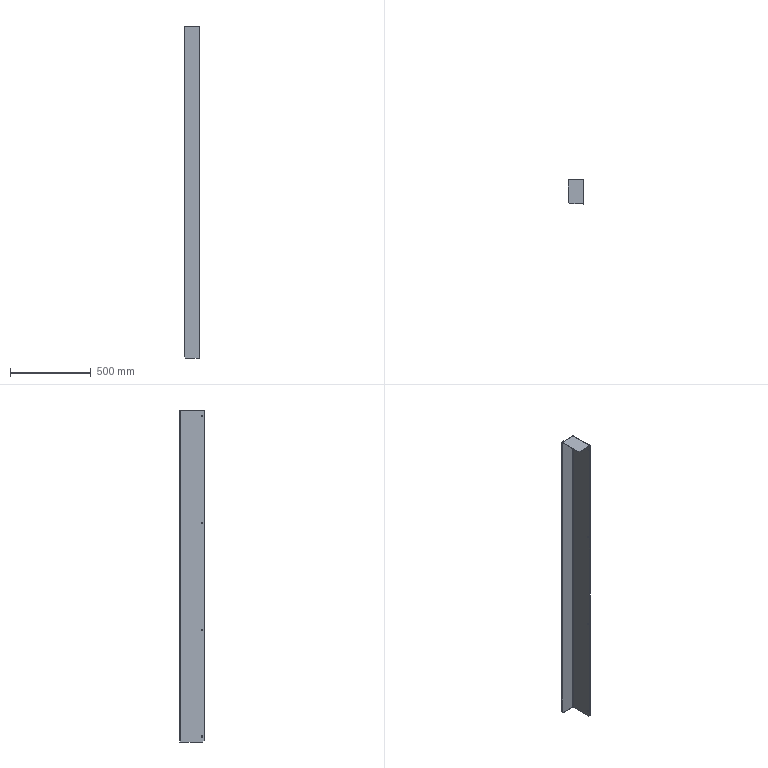Part | STEP file | HXGR200008-05-04 | 2 solids | 32 faces | box 98 x 150 x 2052 mm | volume 1030227 mm3 | plane 22 | cylinder 10 | commonest cylinder face diameters 8 x8 6 x1 10 x1
STEP:
#1=CARTESIAN_POINT('',(96.,-136.,332.));
#2=VERTEX_POINT('',#1);
#3=CARTESIAN_POINT('',(96.,-136.,324.));
#4=VERTEX_POINT('',#3);
#5=CARTESIAN_POINT('',(96.,-136.,328.));
#6=DIRECTION('',(1.,0.,0.));
#7=DIRECTION('',(0.,1.,0.));
#8=AXIS2_PLACEMENT_3D('',#5,#6,#7);
#9=CIRCLE('',#8,4.);
#10=EDGE_CURVE('',#2,#4,#9,.T.);
#11=ORIENTED_EDGE('',*,*,#10,.F.);
#12=CARTESIAN_POINT('',(98.,-136.,332.));
#13=VERTEX_POINT('',#12);
#14=CARTESIAN_POINT('',(98.,-136.,332.));
#15=DIRECTION('',(1.,0.,0.));
#16=VECTOR('',#15,1000.);
#17=LINE('',#14,#16);
#18=EDGE_CURVE('',#2,#13,#17,.T.);
#19=ORIENTED_EDGE('',*,*,#18,.T.);
#20=CARTESIAN_POINT('',(98.,-136.,324.));
#21=VERTEX_POINT('',#20);
#22=CARTESIAN_POINT('',(98.,-136.,328.));
#23=DIRECTION('',(1.,0.,0.));
#24=DIRECTION('',(0.,0.,-1.));
#25=AXIS2_PLACEMENT_3D('',#22,#23,#24);
#26=CIRCLE('',#25,4.);
#27=EDGE_CURVE('',#13,#21,#26,.T.);
#28=ORIENTED_EDGE('',*,*,#27,.T.);
#29=CARTESIAN_POINT('',(98.,-136.,324.));
#30=DIRECTION('',(1.,0.,0.));
#31=VECTOR('',#30,1000.);
#32=LINE('',#29,#31);
#33=EDGE_CURVE('',#4,#21,#32,.T.);
#34=ORIENTED_EDGE('',*,*,#33,.F.);
#35=EDGE_LOOP('',(#11,#19,#28,#34));
#36=FACE_OUTER_BOUND('',#35,.T.);
#37=CARTESIAN_POINT('',(98.,-136.,328.));
#38=DIRECTION('',(1.,0.,0.));
#39=DIRECTION('',(0.,0.,-1.));
#40=AXIS2_PLACEMENT_3D('',#37,#38,#39);
#41=CYLINDRICAL_SURFACE('',#40,4.);
#42=ADVANCED_FACE('',(#36),#41,.F.);
#43=CARTESIAN_POINT('',(96.,-136.,-328.));
#44=VERTEX_POINT('',#43);
#45=CARTESIAN_POINT('',(96.,-136.,-336.));
#46=VERTEX_POINT('',#45);
#47=CARTESIAN_POINT('',(96.,-136.,-332.));
#48=DIRECTION('',(1.,0.,0.));
#49=DIRECTION('',(0.,1.,0.));
#50=AXIS2_PLACEMENT_3D('',#47,#48,#49);
#51=CIRCLE('',#50,4.);
#52=EDGE_CURVE('',#44,#46,#51,.T.);
#53=ORIENTED_EDGE('',*,*,#52,.F.);
#54=CARTESIAN_POINT('',(98.,-136.,-328.));
#55=VERTEX_POINT('',#54);
#56=CARTESIAN_POINT('',(98.,-136.,-328.));
#57=DIRECTION('',(1.,0.,0.));
#58=VECTOR('',#57,1000.);
#59=LINE('',#56,#58);
#60=EDGE_CURVE('',#44,#55,#59,.T.);
#61=ORIENTED_EDGE('',*,*,#60,.T.);
#62=CARTESIAN_POINT('',(98.,-136.,-336.));
#63=VERTEX_POINT('',#62);
#64=CARTESIAN_POINT('',(98.,-136.,-332.));
#65=DIRECTION('',(1.,0.,0.));
#66=DIRECTION('',(0.,0.,-1.));
#67=AXIS2_PLACEMENT_3D('',#64,#65,#66);
#68=CIRCLE('',#67,4.);
#69=EDGE_CURVE('',#55,#63,#68,.T.);
#70=ORIENTED_EDGE('',*,*,#69,.T.);
#71=CARTESIAN_POINT('',(98.,-136.,-336.));
#72=DIRECTION('',(1.,0.,0.));
#73=VECTOR('',#72,1000.);
#74=LINE('',#71,#73);
#75=EDGE_CURVE('',#46,#63,#74,.T.);
#76=ORIENTED_EDGE('',*,*,#75,.F.);
#77=EDGE_LOOP('',(#53,#61,#70,#76));
#78=FACE_OUTER_BOUND('',#77,.T.);
#79=CARTESIAN_POINT('',(98.,-136.,-332.));
#80=DIRECTION('',(1.,0.,0.));
#81=DIRECTION('',(0.,0.,-1.));
#82=AXIS2_PLACEMENT_3D('',#79,#80,#81);
#83=CYLINDRICAL_SURFACE('',#82,4.);
#84=ADVANCED_FACE('',(#78),#83,.F.);
#85=CARTESIAN_POINT('',(96.,-136.,-988.));
#86=VERTEX_POINT('',#85);
#87=CARTESIAN_POINT('',(96.,-136.,-996.));
#88=VERTEX_POINT('',#87);
#89=CARTESIAN_POINT('',(96.,-136.,-992.));
#90=DIRECTION('',(1.,0.,0.));
#91=DIRECTION('',(0.,1.,0.));
#92=AXIS2_PLACEMENT_3D('',#89,#90,#91);
#93=CIRCLE('',#92,4.);
#94=EDGE_CURVE('',#86,#88,#93,.T.);
#95=ORIENTED_EDGE('',*,*,#94,.F.);
#96=CARTESIAN_POINT('',(98.,-136.,-988.));
#97=VERTEX_POINT('',#96);
#98=CARTESIAN_POINT('',(98.,-136.,-988.));
#99=DIRECTION('',(1.,0.,0.));
#100=VECTOR('',#99,1000.);
#101=LINE('',#98,#100);
#102=EDGE_CURVE('',#86,#97,#101,.T.);
#103=ORIENTED_EDGE('',*,*,#102,.T.);
#104=CARTESIAN_POINT('',(98.,-136.,-996.));
#105=VERTEX_POINT('',#104);
#106=CARTESIAN_POINT('',(98.,-136.,-992.));
#107=DIRECTION('',(1.,0.,0.));
#108=DIRECTION('',(0.,0.,-1.));
#109=AXIS2_PLACEMENT_3D('',#106,#107,#108);
#110=CIRCLE('',#109,4.);
#111=EDGE_CURVE('',#97,#105,#110,.T.);
#112=ORIENTED_EDGE('',*,*,#111,.T.);
#113=CARTESIAN_POINT('',(98.,-136.,-996.));
#114=DIRECTION('',(1.,0.,0.));
#115=VECTOR('',#114,1000.);
#116=LINE('',#113,#115);
#117=EDGE_CURVE('',#88,#105,#116,.T.);
#118=ORIENTED_EDGE('',*,*,#117,.F.);
#119=EDGE_LOOP('',(#95,#103,#112,#118));
#120=FACE_OUTER_BOUND('',#119,.T.);
#121=CARTESIAN_POINT('',(98.,-136.,-992.));
#122=DIRECTION('',(1.,0.,0.));
#123=DIRECTION('',(0.,0.,-1.));
#124=AXIS2_PLACEMENT_3D('',#121,#122,#123);
#125=CYLINDRICAL_SURFACE('',#124,4.);
#126=ADVANCED_FACE('',(#120),#125,.F.);
#127=CARTESIAN_POINT('',(96.,-136.,992.));
#128=VERTEX_POINT('',#127);
#129=CARTESIAN_POINT('',(96.,-136.,984.));
#130=VERTEX_POINT('',#129);
#131=CARTESIAN_POINT('',(96.,-136.,988.));
#132=DIRECTION('',(1.,0.,0.));
#133=DIRECTION('',(0.,1.,0.));
#134=AXIS2_PLACEMENT_3D('',#131,#132,#133);
#135=CIRCLE('',#134,4.);
#136=EDGE_CURVE('',#128,#130,#135,.T.);
#137=ORIENTED_EDGE('',*,*,#136,.F.);
#138=CARTESIAN_POINT('',(98.,-136.,992.));
#139=VERTEX_POINT('',#138);
#140=CARTESIAN_POINT('',(98.,-136.,992.));
#141=DIRECTION('',(1.,0.,0.));
#142=VECTOR('',#141,1000.);
#143=LINE('',#140,#142);
#144=EDGE_CURVE('',#128,#139,#143,.T.);
#145=ORIENTED_EDGE('',*,*,#144,.T.);
#146=CARTESIAN_POINT('',(98.,-136.,984.));
#147=VERTEX_POINT('',#146);
#148=CARTESIAN_POINT('',(98.,-136.,988.));
#149=DIRECTION('',(1.,0.,0.));
#150=DIRECTION('',(0.,0.,-1.));
#151=AXIS2_PLACEMENT_3D('',#148,#149,#150);
#152=CIRCLE('',#151,4.);
#153=EDGE_CURVE('',#139,#147,#152,.T.);
#154=ORIENTED_EDGE('',*,*,#153,.T.);
#155=CARTESIAN_POINT('',(98.,-136.,984.));
#156=DIRECTION('',(1.,0.,0.));
#157=VECTOR('',#156,1000.);
#158=LINE('',#155,#157);
#159=EDGE_CURVE('',#130,#147,#158,.T.);
#160=ORIENTED_EDGE('',*,*,#159,.F.);
#161=EDGE_LOOP('',(#137,#145,#154,#160));
#162=FACE_OUTER_BOUND('',#161,.T.);
#163=CARTESIAN_POINT('',(98.,-136.,988.));
#164=DIRECTION('',(1.,0.,0.));
#165=DIRECTION('',(0.,0.,-1.));
#166=AXIS2_PLACEMENT_3D('',#163,#164,#165);
#167=CYLINDRICAL_SURFACE('',#166,4.);
#168=ADVANCED_FACE('',(#162),#167,.F.);
#169=CARTESIAN_POINT('',(98.,-5.,1026.));
#170=VERTEX_POINT('',#169);
#171=CARTESIAN_POINT('',(96.,-5.,1026.));
#172=VERTEX_POINT('',#171);
#173=CARTESIAN_POINT('',(98.,-5.,1026.));
#174=DIRECTION('',(-1.,0.,0.));
#175=VECTOR('',#174,1000.);
#176=LINE('',#173,#175);
#177=EDGE_CURVE('',#170,#172,#176,.T.);
#178=ORIENTED_EDGE('',*,*,#177,.F.);
#179=CARTESIAN_POINT('',(93.,0.,1026.));
#180=VERTEX_POINT('',#179);
#181=CARTESIAN_POINT('',(93.,-5.,1026.));
#182=DIRECTION('',(0.,0.,-1.));
#183=DIRECTION('',(1.,0.,0.));
#184=AXIS2_PLACEMENT_3D('',#181,#182,#183);
#185=CIRCLE('',#184,5.);
#186=EDGE_CURVE('',#180,#170,#185,.T.);
#187=ORIENTED_EDGE('',*,*,#186,.F.);
#188=CARTESIAN_POINT('',(93.,-2.,1026.));
#189=VERTEX_POINT('',#188);
#190=CARTESIAN_POINT('',(93.,-2.,1026.));
#191=DIRECTION('',(0.,1.,0.));
#192=VECTOR('',#191,1000.);
#193=LINE('',#190,#192);
#194=EDGE_CURVE('',#189,#180,#193,.T.);
#195=ORIENTED_EDGE('',*,*,#194,.F.);
#196=CARTESIAN_POINT('',(93.,-5.,1026.));
#197=DIRECTION('',(0.,0.,-1.));
#198=DIRECTION('',(1.,0.,0.));
#199=AXIS2_PLACEMENT_3D('',#196,#197,#198);
#200=CIRCLE('',#199,3.);
#201=EDGE_CURVE('',#189,#172,#200,.T.);
#202=ORIENTED_EDGE('',*,*,#201,.T.);
#203=EDGE_LOOP('',(#178,#187,#195,#202));
#204=FACE_OUTER_BOUND('',#203,.T.);
#205=CARTESIAN_POINT('',(98.,-5.,1026.));
#206=DIRECTION('',(0.,0.,1.));
#207=DIRECTION('',(1.,0.,0.));
#208=AXIS2_PLACEMENT_3D('',#205,#206,#207);
#209=PLANE('',#208);
#210=ADVANCED_FACE('',(#204),#209,.T.);
#211=CARTESIAN_POINT('',(98.,-150.,1026.));
#212=VERTEX_POINT('',#211);
#213=CARTESIAN_POINT('',(98.,0.,1026.));
#214=DIRECTION('',(0.,-1.,0.));
#215=VECTOR('',#214,1000.);
#216=LINE('',#213,#215);
#217=EDGE_CURVE('',#170,#212,#216,.T.);
#218=ORIENTED_EDGE('',*,*,#217,.F.);
#219=ORIENTED_EDGE('',*,*,#177,.T.);
#220=CARTESIAN_POINT('',(96.,-150.,1026.));
#221=VERTEX_POINT('',#220);
#222=CARTESIAN_POINT('',(96.,0.,1026.));
#223=DIRECTION('',(0.,-1.,0.));
#224=VECTOR('',#223,1000.);
#225=LINE('',#222,#224);
#226=EDGE_CURVE('',#172,#221,#225,.T.);
#227=ORIENTED_EDGE('',*,*,#226,.T.);
#228=CARTESIAN_POINT('',(98.,-150.,1026.));
#229=DIRECTION('',(-1.,0.,0.));
#230=VECTOR('',#229,1000.);
#231=LINE('',#228,#230);
#232=EDGE_CURVE('',#212,#221,#231,.T.);
#233=ORIENTED_EDGE('',*,*,#232,.F.);
#234=EDGE_LOOP('',(#218,#219,#227,#233));
#235=FACE_OUTER_BOUND('',#234,.T.);
#236=CARTESIAN_POINT('',(93.,-2.,1026.));
#237=DIRECTION('',(0.,0.,1.));
#238=DIRECTION('',(1.,0.,0.));
#239=AXIS2_PLACEMENT_3D('',#236,#237,#238);
#240=PLANE('',#239);
#241=ADVANCED_FACE('',(#235),#240,.T.);
#242=CARTESIAN_POINT('',(93.,0.,-1026.));
#243=VERTEX_POINT('',#242);
#244=CARTESIAN_POINT('',(93.,-2.,-1026.));
#245=VERTEX_POINT('',#244);
#246=CARTESIAN_POINT('',(93.,0.,-1026.));
#247=DIRECTION('',(0.,-1.,0.));
#248=VECTOR('',#247,1000.);
#249=LINE('',#246,#248);
#250=EDGE_CURVE('',#243,#245,#249,.T.);
#251=ORIENTED_EDGE('',*,*,#250,.F.);
#252=CARTESIAN_POINT('',(98.,-5.,-1026.));
#253=VERTEX_POINT('',#252);
#254=CARTESIAN_POINT('',(93.,-5.,-1026.));
#255=DIRECTION('',(0.,0.,-1.));
#256=DIRECTION('',(1.,0.,0.));
#257=AXIS2_PLACEMENT_3D('',#254,#255,#256);
#258=CIRCLE('',#257,5.);
#259=EDGE_CURVE('',#243,#253,#258,.T.);
#260=ORIENTED_EDGE('',*,*,#259,.T.);
#261=CARTESIAN_POINT('',(96.,-5.,-1026.));
#262=VERTEX_POINT('',#261);
#263=CARTESIAN_POINT('',(96.,-5.,-1026.));
#264=DIRECTION('',(1.,0.,0.));
#265=VECTOR('',#264,1000.);
#266=LINE('',#263,#265);
#267=EDGE_CURVE('',#262,#253,#266,.T.);
#268=ORIENTED_EDGE('',*,*,#267,.F.);
#269=CARTESIAN_POINT('',(93.,-5.,-1026.));
#270=DIRECTION('',(0.,0.,-1.));
#271=DIRECTION('',(1.,0.,0.));
#272=AXIS2_PLACEMENT_3D('',#269,#270,#271);
#273=CIRCLE('',#272,3.);
#274=EDGE_CURVE('',#245,#262,#273,.T.);
#275=ORIENTED_EDGE('',*,*,#274,.F.);
#276=EDGE_LOOP('',(#251,#260,#268,#275));
#277=FACE_OUTER_BOUND('',#276,.T.);
#278=CARTESIAN_POINT('',(93.,0.,-1026.));
#279=DIRECTION('',(0.,0.,-1.));
#280=DIRECTION('',(-1.,0.,0.));
#281=AXIS2_PLACEMENT_3D('',#278,#279,#280);
#282=PLANE('',#281);
#283=ADVANCED_FACE('',(#277),#282,.T.);
#284=CARTESIAN_POINT('',(10.,-2.,-1026.));
#285=VERTEX_POINT('',#284);
#286=CARTESIAN_POINT('',(0.,-2.,-1026.));
#287=DIRECTION('',(1.,0.,0.));
#288=VECTOR('',#287,1000.);
#289=LINE('',#286,#288);
#290=EDGE_CURVE('',#285,#245,#289,.T.);
#291=ORIENTED_EDGE('',*,*,#290,.F.);
#292=CARTESIAN_POINT('',(10.,0.,-1026.));
#293=VERTEX_POINT('',#292);
#294=CARTESIAN_POINT('',(10.,-5.,-1026.));
#295=DIRECTION('',(0.,1.,0.));
#296=VECTOR('',#295,1000.);
#297=LINE('',#294,#296);
#298=EDGE_CURVE('',#285,#293,#297,.T.);
#299=ORIENTED_EDGE('',*,*,#298,.T.);
#300=CARTESIAN_POINT('',(0.,0.,-1026.));
#301=DIRECTION('',(1.,0.,0.));
#302=VECTOR('',#301,1000.);
#303=LINE('',#300,#302);
#304=EDGE_CURVE('',#293,#243,#303,.T.);
#305=ORIENTED_EDGE('',*,*,#304,.T.);
#306=ORIENTED_EDGE('',*,*,#250,.T.);
#307=EDGE_LOOP('',(#291,#299,#305,#306));
#308=FACE_OUTER_BOUND('',#307,.T.);
#309=CARTESIAN_POINT('',(96.,-5.,-1026.));
#310=DIRECTION('',(0.,0.,-1.));
#311=DIRECTION('',(-1.,0.,0.));
#312=AXIS2_PLACEMENT_3D('',#309,#310,#311);
#313=PLANE('',#312);
#314=ADVANCED_FACE('',(#308),#313,.T.);
#315=CARTESIAN_POINT('',(96.,-136.,328.));
#316=DIRECTION('',(1.,0.,0.));
#317=DIRECTION('',(0.,1.,0.));
#318=AXIS2_PLACEMENT_3D('',#315,#316,#317);
#319=CIRCLE('',#318,4.);
#320=EDGE_CURVE('',#4,#2,#319,.T.);
#321=ORIENTED_EDGE('',*,*,#320,.T.);
#322=ORIENTED_EDGE('',*,*,#10,.T.);
#323=EDGE_LOOP('',(#321,#322));
#324=FACE_BOUND('',#323,.T.);
#325=CARTESIAN_POINT('',(96.,-136.,-332.));
#326=DIRECTION('',(1.,0.,0.));
#327=DIRECTION('',(0.,1.,0.));
#328=AXIS2_PLACEMENT_3D('',#325,#326,#327);
#329=CIRCLE('',#328,4.);
#330=EDGE_CURVE('',#46,#44,#329,.T.);
#331=ORIENTED_EDGE('',*,*,#330,.T.);
#332=ORIENTED_EDGE('',*,*,#52,.T.);
#333=EDGE_LOOP('',(#331,#332));
#334=FACE_BOUND('',#333,.T.);
#335=CARTESIAN_POINT('',(96.,-136.,-992.));
#336=DIRECTION('',(1.,0.,0.));
#337=DIRECTION('',(0.,1.,0.));
#338=AXIS2_PLACEMENT_3D('',#335,#336,#337);
#339=CIRCLE('',#338,4.);
#340=EDGE_CURVE('',#88,#86,#339,.T.);
#341=ORIENTED_EDGE('',*,*,#340,.T.);
#342=ORIENTED_EDGE('',*,*,#94,.T.);
#343=EDGE_LOOP('',(#341,#342));
#344=FACE_BOUND('',#343,.T.);
#345=CARTESIAN_POINT('',(96.,-136.,988.));
#346=DIRECTION('',(1.,0.,0.));
#347=DIRECTION('',(0.,1.,0.));
#348=AXIS2_PLACEMENT_3D('',#345,#346,#347);
#349=CIRCLE('',#348,4.);
#350=EDGE_CURVE('',#130,#128,#349,.T.);
#351=ORIENTED_EDGE('',*,*,#350,.T.);
#352=ORIENTED_EDGE('',*,*,#136,.T.);
#353=EDGE_LOOP('',(#351,#352));
#354=FACE_BOUND('',#353,.T.);
#355=CARTESIAN_POINT('',(96.,-140.,-1026.));
#356=VERTEX_POINT('',#355);
#357=CARTESIAN_POINT('',(96.,0.,-1026.));
#358=DIRECTION('',(0.,-1.,0.));
#359=VECTOR('',#358,1000.);
#360=LINE('',#357,#359);
#361=EDGE_CURVE('',#262,#356,#360,.T.);
#362=ORIENTED_EDGE('',*,*,#361,.T.);
#363=CARTESIAN_POINT('',(96.,-150.,-1016.));
#364=VERTEX_POINT('',#363);
#365=CARTESIAN_POINT('',(96.,-140.,-1026.));
#366=DIRECTION('',(0.,-0.7071,0.7071));
#367=VECTOR('',#366,1000.);
#368=LINE('',#365,#367);
#369=EDGE_CURVE('',#356,#364,#368,.T.);
#370=ORIENTED_EDGE('',*,*,#369,.T.);
#371=CARTESIAN_POINT('',(96.,-150.,1026.));
#372=DIRECTION('',(0.,0.,-1.));
#373=VECTOR('',#372,1000.);
#374=LINE('',#371,#373);
#375=EDGE_CURVE('',#221,#364,#374,.T.);
#376=ORIENTED_EDGE('',*,*,#375,.F.);
#377=ORIENTED_EDGE('',*,*,#226,.F.);
#378=CARTESIAN_POINT('',(96.,-5.,1026.));
#379=DIRECTION('',(0.,0.,-1.));
#380=VECTOR('',#379,1000.);
#381=LINE('',#378,#380);
#382=EDGE_CURVE('',#172,#262,#381,.T.);
#383=ORIENTED_EDGE('',*,*,#382,.T.);
#384=EDGE_LOOP('',(#362,#370,#376,#377,#383));
#385=FACE_OUTER_BOUND('',#384,.T.);
#386=CARTESIAN_POINT('',(96.,0.,1026.));
#387=DIRECTION('',(1.,0.,0.));
#388=DIRECTION('',(0.,1.,0.));
#389=AXIS2_PLACEMENT_3D('',#386,#387,#388);
#390=PLANE('',#389);
#391=ADVANCED_FACE('',(#324,#334,#344,#354,#385),#390,.F.);
#392=ORIENTED_EDGE('',*,*,#375,.T.);
#393=CARTESIAN_POINT('',(98.,-150.,-1016.));
#394=VERTEX_POINT('',#393);
#395=CARTESIAN_POINT('',(98.,-150.,-1016.));
#396=DIRECTION('',(1.,0.,0.));
#397=VECTOR('',#396,1000.);
#398=LINE('',#395,#397);
#399=EDGE_CURVE('',#364,#394,#398,.T.);
#400=ORIENTED_EDGE('',*,*,#399,.T.);
#401=CARTESIAN_POINT('',(98.,-150.,1026.));
#402=DIRECTION('',(0.,0.,-1.));
#403=VECTOR('',#402,1000.);
#404=LINE('',#401,#403);
#405=EDGE_CURVE('',#212,#394,#404,.T.);
#406=ORIENTED_EDGE('',*,*,#405,.F.);
#407=ORIENTED_EDGE('',*,*,#232,.T.);
#408=EDGE_LOOP('',(#392,#400,#406,#407));
#409=FACE_OUTER_BOUND('',#408,.T.);
#410=CARTESIAN_POINT('',(98.,-150.,1026.));
#411=DIRECTION('',(0.,-1.,0.));
#412=DIRECTION('',(0.,0.,-1.));
#413=AXIS2_PLACEMENT_3D('',#410,#411,#412);
#414=PLANE('',#413);
#415=ADVANCED_FACE('',(#409),#414,.T.);
#416=CARTESIAN_POINT('',(98.,-136.,328.));
#417=DIRECTION('',(1.,0.,0.));
#418=DIRECTION('',(0.,0.,-1.));
#419=AXIS2_PLACEMENT_3D('',#416,#417,#418);
#420=CIRCLE('',#419,4.);
#421=EDGE_CURVE('',#21,#13,#420,.T.);
#422=ORIENTED_EDGE('',*,*,#421,.F.);
#423=ORIENTED_EDGE('',*,*,#27,.F.);
#424=EDGE_LOOP('',(#422,#423));
#425=FACE_BOUND('',#424,.T.);
#426=CARTESIAN_POINT('',(98.,-136.,-332.));
#427=DIRECTION('',(1.,0.,0.));
#428=DIRECTION('',(0.,0.,-1.));
#429=AXIS2_PLACEMENT_3D('',#426,#427,#428);
#430=CIRCLE('',#429,4.);
#431=EDGE_CURVE('',#63,#55,#430,.T.);
#432=ORIENTED_EDGE('',*,*,#431,.F.);
#433=ORIENTED_EDGE('',*,*,#69,.F.);
#434=EDGE_LOOP('',(#432,#433));
#435=FACE_BOUND('',#434,.T.);
#436=CARTESIAN_POINT('',(98.,-136.,-992.));
#437=DIRECTION('',(1.,0.,0.));
#438=DIRECTION('',(0.,0.,-1.));
#439=AXIS2_PLACEMENT_3D('',#436,#437,#438);
#440=CIRCLE('',#439,4.);
#441=EDGE_CURVE('',#105,#97,#440,.T.);
#442=ORIENTED_EDGE('',*,*,#441,.F.);
#443=ORIENTED_EDGE('',*,*,#111,.F.);
#444=EDGE_LOOP('',(#442,#443));
#445=FACE_BOUND('',#444,.T.);
#446=CARTESIAN_POINT('',(98.,-136.,988.));
#447=DIRECTION('',(1.,0.,0.));
#448=DIRECTION('',(0.,0.,-1.));
#449=AXIS2_PLACEMENT_3D('',#446,#447,#448);
#450=CIRCLE('',#449,4.);
#451=EDGE_CURVE('',#147,#139,#450,.T.);
#452=ORIENTED_EDGE('',*,*,#451,.F.);
#453=ORIENTED_EDGE('',*,*,#153,.F.);
#454=EDGE_LOOP('',(#452,#453));
#455=FACE_BOUND('',#454,.T.);
#456=ORIENTED_EDGE('',*,*,#405,.T.);
#457=CARTESIAN_POINT('',(98.,-140.,-1026.));
#458=VERTEX_POINT('',#457);
#459=CARTESIAN_POINT('',(98.,-1096.,-70.));
#460=DIRECTION('',(0.,0.7071,-0.7071));
#461=VECTOR('',#460,1000.);
#462=LINE('',#459,#461);
#463=EDGE_CURVE('',#394,#458,#462,.T.);
#464=ORIENTED_EDGE('',*,*,#463,.T.);
#465=CARTESIAN_POINT('',(98.,0.,-1026.));
#466=DIRECTION('',(0.,-1.,0.));
#467=VECTOR('',#466,1000.);
#468=LINE('',#465,#467);
#469=EDGE_CURVE('',#253,#458,#468,.T.);
#470=ORIENTED_EDGE('',*,*,#469,.F.);
#471=CARTESIAN_POINT('',(98.,-5.,1026.));
#472=DIRECTION('',(0.,0.,-1.));
#473=VECTOR('',#472,1000.);
#474=LINE('',#471,#473);
#475=EDGE_CURVE('',#170,#253,#474,.T.);
#476=ORIENTED_EDGE('',*,*,#475,.F.);
#477=ORIENTED_EDGE('',*,*,#217,.T.);
#478=EDGE_LOOP('',(#456,#464,#470,#476,#477));
#479=FACE_OUTER_BOUND('',#478,.T.);
#480=CARTESIAN_POINT('',(98.,0.,1026.));
#481=DIRECTION('',(1.,0.,0.));
#482=DIRECTION('',(0.,1.,0.));
#483=AXIS2_PLACEMENT_3D('',#480,#481,#482);
#484=PLANE('',#483);
#485=ADVANCED_FACE('',(#425,#435,#445,#455,#479),#484,.T.);
#486=ORIENTED_EDGE('',*,*,#259,.F.);
#487=CARTESIAN_POINT('',(93.,0.,1026.));
#488=DIRECTION('',(0.,0.,-1.));
#489=VECTOR('',#488,1000.);
#490=LINE('',#487,#489);
#491=EDGE_CURVE('',#180,#243,#490,.T.);
#492=ORIENTED_EDGE('',*,*,#491,.F.);
#493=ORIENTED_EDGE('',*,*,#186,.T.);
#494=ORIENTED_EDGE('',*,*,#475,.T.);
#495=EDGE_LOOP('',(#486,#492,#493,#494));
#496=FACE_OUTER_BOUND('',#495,.T.);
#497=CARTESIAN_POINT('',(93.,-5.,1026.));
#498=DIRECTION('',(0.,0.,-1.));
#499=DIRECTION('',(-1.,0.,0.));
#500=AXIS2_PLACEMENT_3D('',#497,#498,#499);
#501=CYLINDRICAL_SURFACE('',#500,5.);
#502=ADVANCED_FACE('',(#496),#501,.T.);
#503=ORIENTED_EDGE('',*,*,#304,.F.);
#504=CARTESIAN_POINT('',(0.,0.,-1016.));
#505=VERTEX_POINT('',#504);
#506=CARTESIAN_POINT('',(-1021.,0.,5.));
#507=DIRECTION('',(-0.7071,0.,0.7071));
#508=VECTOR('',#507,1000.);
#509=LINE('',#506,#508);
#510=EDGE_CURVE('',#293,#505,#509,.T.);
#511=ORIENTED_EDGE('',*,*,#510,.T.);
#512=CARTESIAN_POINT('',(0.,0.,1026.));
#513=VERTEX_POINT('',#512);
#514=CARTESIAN_POINT('',(0.,0.,1026.));
#515=DIRECTION('',(0.,0.,-1.));
#516=VECTOR('',#515,1000.);
#517=LINE('',#514,#516);
#518=EDGE_CURVE('',#513,#505,#517,.T.);
#519=ORIENTED_EDGE('',*,*,#518,.F.);
#520=CARTESIAN_POINT('',(0.,0.,1026.));
#521=DIRECTION('',(1.,0.,0.));
#522=VECTOR('',#521,1000.);
#523=LINE('',#520,#522);
#524=EDGE_CURVE('',#513,#180,#523,.T.);
#525=ORIENTED_EDGE('',*,*,#524,.T.);
#526=ORIENTED_EDGE('',*,*,#491,.T.);
#527=EDGE_LOOP('',(#503,#511,#519,#525,#526));
#528=FACE_OUTER_BOUND('',#527,.T.);
#529=CARTESIAN_POINT('',(0.,0.,1026.));
#530=DIRECTION('',(0.,1.,0.));
#531=DIRECTION('',(0.,0.,1.));
#532=AXIS2_PLACEMENT_3D('',#529,#530,#531);
#533=PLANE('',#532);
#534=ADVANCED_FACE('',(#528),#533,.T.);
#535=ORIENTED_EDGE('',*,*,#518,.T.);
#536=CARTESIAN_POINT('',(0.,-2.,-1016.));
#537=VERTEX_POINT('',#536);
#538=CARTESIAN_POINT('',(0.,-2.,-1016.));
#539=DIRECTION('',(0.,-1.,0.));
#540=VECTOR('',#539,1000.);
#541=LINE('',#538,#540);
#542=EDGE_CURVE('',#505,#537,#541,.T.);
#543=ORIENTED_EDGE('',*,*,#542,.T.);
#544=CARTESIAN_POINT('',(0.,-2.,1026.));
#545=VERTEX_POINT('',#544);
#546=CARTESIAN_POINT('',(0.,-2.,1026.));
#547=DIRECTION('',(0.,0.,-1.));
#548=VECTOR('',#547,1000.);
#549=LINE('',#546,#548);
#550=EDGE_CURVE('',#545,#537,#549,.T.);
#551=ORIENTED_EDGE('',*,*,#550,.F.);
#552=CARTESIAN_POINT('',(0.,-2.,1026.));
#553=DIRECTION('',(0.,1.,0.));
#554=VECTOR('',#553,1000.);
#555=LINE('',#552,#554);
#556=EDGE_CURVE('',#545,#513,#555,.T.);
#557=ORIENTED_EDGE('',*,*,#556,.T.);
#558=EDGE_LOOP('',(#535,#543,#551,#557));
#559=FACE_OUTER_BOUND('',#558,.T.);
#560=CARTESIAN_POINT('',(0.,-2.,1026.));
#561=DIRECTION('',(-1.,0.,0.));
#562=DIRECTION('',(0.,0.,1.));
#563=AXIS2_PLACEMENT_3D('',#560,#561,#562);
#564=PLANE('',#563);
#565=ADVANCED_FACE('',(#559),#564,.T.);
#566=ORIENTED_EDGE('',*,*,#550,.T.);
#567=CARTESIAN_POINT('',(10.,-2.,-1026.));
#568=DIRECTION('',(0.7071,0.,-0.7071));
#569=VECTOR('',#568,1000.);
#570=LINE('',#567,#569);
#571=EDGE_CURVE('',#537,#285,#570,.T.);
#572=ORIENTED_EDGE('',*,*,#571,.T.);
#573=ORIENTED_EDGE('',*,*,#290,.T.);
#574=CARTESIAN_POINT('',(93.,-2.,1026.));
#575=DIRECTION('',(0.,0.,-1.));
#576=VECTOR('',#575,1000.);
#577=LINE('',#574,#576);
#578=EDGE_CURVE('',#189,#245,#577,.T.);
#579=ORIENTED_EDGE('',*,*,#578,.F.);
#580=CARTESIAN_POINT('',(0.,-2.,1026.));
#581=DIRECTION('',(1.,0.,0.));
#582=VECTOR('',#581,1000.);
#583=LINE('',#580,#582);
#584=EDGE_CURVE('',#545,#189,#583,.T.);
#585=ORIENTED_EDGE('',*,*,#584,.F.);
#586=EDGE_LOOP('',(#566,#572,#573,#579,#585));
#587=FACE_OUTER_BOUND('',#586,.T.);
#588=CARTESIAN_POINT('',(0.,-2.,1026.));
#589=DIRECTION('',(0.,1.,0.));
#590=DIRECTION('',(0.,0.,1.));
#591=AXIS2_PLACEMENT_3D('',#588,#589,#590);
#592=PLANE('',#591);
#593=ADVANCED_FACE('',(#587),#592,.F.);
#594=ORIENTED_EDGE('',*,*,#274,.T.);
#595=ORIENTED_EDGE('',*,*,#382,.F.);
#596=ORIENTED_EDGE('',*,*,#201,.F.);
#597=ORIENTED_EDGE('',*,*,#578,.T.);
#598=EDGE_LOOP('',(#594,#595,#596,#597));
#599=FACE_OUTER_BOUND('',#598,.T.);
#600=CARTESIAN_POINT('',(93.,-5.,1026.));
#601=DIRECTION('',(0.,0.,-1.));
#602=DIRECTION('',(-1.,0.,0.));
#603=AXIS2_PLACEMENT_3D('',#600,#601,#602);
#604=CYLINDRICAL_SURFACE('',#603,3.);
#605=ADVANCED_FACE('',(#599),#604,.F.);
#606=ORIENTED_EDGE('',*,*,#584,.T.);
#607=ORIENTED_EDGE('',*,*,#194,.T.);
#608=ORIENTED_EDGE('',*,*,#524,.F.);
#609=ORIENTED_EDGE('',*,*,#556,.F.);
#610=EDGE_LOOP('',(#606,#607,#608,#609));
#611=FACE_OUTER_BOUND('',#610,.T.);
#612=CARTESIAN_POINT('',(93.,-5.,1026.));
#613=DIRECTION('',(0.,0.,1.));
#614=DIRECTION('',(1.,0.,0.));
#615=AXIS2_PLACEMENT_3D('',#612,#613,#614);
#616=PLANE('',#615);
#617=ADVANCED_FACE('',(#611),#616,.T.);
#618=ORIENTED_EDGE('',*,*,#469,.T.);
#619=CARTESIAN_POINT('',(96.,-140.,-1026.));
#620=DIRECTION('',(-1.,0.,0.));
#621=VECTOR('',#620,1000.);
#622=LINE('',#619,#621);
#623=EDGE_CURVE('',#458,#356,#622,.T.);
#624=ORIENTED_EDGE('',*,*,#623,.T.);
#625=ORIENTED_EDGE('',*,*,#361,.F.);
#626=ORIENTED_EDGE('',*,*,#267,.T.);
#627=EDGE_LOOP('',(#618,#624,#625,#626));
#628=FACE_OUTER_BOUND('',#627,.T.);
#629=CARTESIAN_POINT('',(93.,-5.,-1026.));
#630=DIRECTION('',(0.,0.,1.));
#631=DIRECTION('',(1.,0.,0.));
#632=AXIS2_PLACEMENT_3D('',#629,#630,#631);
#633=PLANE('',#632);
#634=ADVANCED_FACE('',(#628),#633,.F.);
#635=ORIENTED_EDGE('',*,*,#144,.F.);
#636=ORIENTED_EDGE('',*,*,#350,.F.);
#637=ORIENTED_EDGE('',*,*,#159,.T.);
#638=ORIENTED_EDGE('',*,*,#451,.T.);
#639=EDGE_LOOP('',(#635,#636,#637,#638));
#640=FACE_OUTER_BOUND('',#639,.T.);
#641=CARTESIAN_POINT('',(98.,-136.,988.));
#642=DIRECTION('',(1.,0.,0.));
#643=DIRECTION('',(0.,0.,-1.));
#644=AXIS2_PLACEMENT_3D('',#641,#642,#643);
#645=CYLINDRICAL_SURFACE('',#644,4.);
#646=ADVANCED_FACE('',(#640),#645,.F.);
#647=ORIENTED_EDGE('',*,*,#102,.F.);
#648=ORIENTED_EDGE('',*,*,#340,.F.);
#649=ORIENTED_EDGE('',*,*,#117,.T.);
#650=ORIENTED_EDGE('',*,*,#441,.T.);
#651=EDGE_LOOP('',(#647,#648,#649,#650));
#652=FACE_OUTER_BOUND('',#651,.T.);
#653=CARTESIAN_POINT('',(98.,-136.,-992.));
#654=DIRECTION('',(1.,0.,0.));
#655=DIRECTION('',(0.,0.,-1.));
#656=AXIS2_PLACEMENT_3D('',#653,#654,#655);
#657=CYLINDRICAL_SURFACE('',#656,4.);
#658=ADVANCED_FACE('',(#652),#657,.F.);
#659=ORIENTED_EDGE('',*,*,#60,.F.);
#660=ORIENTED_EDGE('',*,*,#330,.F.);
#661=ORIENTED_EDGE('',*,*,#75,.T.);
#662=ORIENTED_EDGE('',*,*,#431,.T.);
#663=EDGE_LOOP('',(#659,#660,#661,#662));
#664=FACE_OUTER_BOUND('',#663,.T.);
#665=CARTESIAN_POINT('',(98.,-136.,-332.));
#666=DIRECTION('',(1.,0.,0.));
#667=DIRECTION('',(0.,0.,-1.));
#668=AXIS2_PLACEMENT_3D('',#665,#666,#667);
#669=CYLINDRICAL_SURFACE('',#668,4.);
#670=ADVANCED_FACE('',(#664),#669,.F.);
#671=ORIENTED_EDGE('',*,*,#18,.F.);
#672=ORIENTED_EDGE('',*,*,#320,.F.);
#673=ORIENTED_EDGE('',*,*,#33,.T.);
#674=ORIENTED_EDGE('',*,*,#421,.T.);
#675=EDGE_LOOP('',(#671,#672,#673,#674));
#676=FACE_OUTER_BOUND('',#675,.T.);
#677=CARTESIAN_POINT('',(98.,-136.,328.));
#678=DIRECTION('',(1.,0.,0.));
#679=DIRECTION('',(0.,0.,-1.));
#680=AXIS2_PLACEMENT_3D('',#677,#678,#679);
#681=CYLINDRICAL_SURFACE('',#680,4.);
#682=ADVANCED_FACE('',(#676),#681,.F.);
#683=ORIENTED_EDGE('',*,*,#463,.F.);
#684=ORIENTED_EDGE('',*,*,#399,.F.);
#685=ORIENTED_EDGE('',*,*,#369,.F.);
#686=ORIENTED_EDGE('',*,*,#623,.F.);
#687=EDGE_LOOP('',(#683,#684,#685,#686));
#688=FACE_OUTER_BOUND('',#687,.T.);
#689=CARTESIAN_POINT('',(93.,-140.,-1026.));
#690=DIRECTION('',(0.,-0.7071,-0.7071));
#691=DIRECTION('',(1.,0.,0.));
#692=AXIS2_PLACEMENT_3D('',#689,#690,#691);
#693=PLANE('',#692);
#694=ADVANCED_FACE('',(#688),#693,.T.);
#695=ORIENTED_EDGE('',*,*,#571,.F.);
#696=ORIENTED_EDGE('',*,*,#542,.F.);
#697=ORIENTED_EDGE('',*,*,#510,.F.);
#698=ORIENTED_EDGE('',*,*,#298,.F.);
#699=EDGE_LOOP('',(#695,#696,#697,#698));
#700=FACE_OUTER_BOUND('',#699,.T.);
#701=CARTESIAN_POINT('',(10.,-5.,-1026.));
#702=DIRECTION('',(0.7071,0.,0.7071));
#703=DIRECTION('',(0.,1.,0.));
#704=AXIS2_PLACEMENT_3D('',#701,#702,#703);
#705=PLANE('',#704);
#706=ADVANCED_FACE('',(#700),#705,.F.);
#707=CLOSED_SHELL('',(#42,#84,#126,#168,#210,#241,#283,#314,#391,#415,#485,#502,#534,#565,#593,#605,#617,#634,#646,#658,#670,#682,#694,#706));
#708=MANIFOLD_SOLID_BREP('',#707);
#709=CARTESIAN_POINT('',(0.,-2.,1026.));
#710=VERTEX_POINT('',#709);
#711=CARTESIAN_POINT('',(0.,-140.,1026.));
#712=VERTEX_POINT('',#711);
#713=CARTESIAN_POINT('',(0.,-2.,1026.));
#714=DIRECTION('',(0.,-1.,0.));
#715=VECTOR('',#714,1000.);
#716=LINE('',#713,#715);
#717=EDGE_CURVE('',#710,#712,#716,.T.);
#718=ORIENTED_EDGE('',*,*,#717,.F.);
#719=CARTESIAN_POINT('',(0.,-2.,1024.));
#720=VERTEX_POINT('',#719);
#721=CARTESIAN_POINT('',(0.,-2.,1024.));
#722=DIRECTION('',(0.,0.,1.));
#723=VECTOR('',#722,1000.);
#724=LINE('',#721,#723);
#725=EDGE_CURVE('',#720,#710,#724,.T.);
#726=ORIENTED_EDGE('',*,*,#725,.F.);
#727=CARTESIAN_POINT('',(0.,-140.,1024.));
#728=VERTEX_POINT('',#727);
#729=CARTESIAN_POINT('',(0.,-2.,1024.));
#730=DIRECTION('',(0.,-1.,0.));
#731=VECTOR('',#730,1000.);
#732=LINE('',#729,#731);
#733=EDGE_CURVE('',#720,#728,#732,.T.);
#734=ORIENTED_EDGE('',*,*,#733,.T.);
#735=CARTESIAN_POINT('',(0.,-140.,1024.));
#736=DIRECTION('',(0.,0.,1.));
#737=VECTOR('',#736,1000.);
#738=LINE('',#735,#737);
#739=EDGE_CURVE('',#728,#712,#738,.T.);
#740=ORIENTED_EDGE('',*,*,#739,.T.);
#741=EDGE_LOOP('',(#718,#726,#734,#740));
#742=FACE_OUTER_BOUND('',#741,.T.);
#743=CARTESIAN_POINT('',(0.,-2.,1024.));
#744=DIRECTION('',(-1.,0.,0.));
#745=DIRECTION('',(0.,-1.,0.));
#746=AXIS2_PLACEMENT_3D('',#743,#744,#745);
#747=PLANE('',#746);
#748=ADVANCED_FACE('',(#742),#747,.T.);
#749=CARTESIAN_POINT('',(91.,-2.,1026.));
#750=VERTEX_POINT('',#749);
#751=CARTESIAN_POINT('',(0.,-2.,1026.));
#752=DIRECTION('',(-1.,0.,0.));
#753=VECTOR('',#752,1000.);
#754=LINE('',#751,#753);
#755=EDGE_CURVE('',#750,#710,#754,.T.);
#756=ORIENTED_EDGE('',*,*,#755,.F.);
#757=CARTESIAN_POINT('',(91.,-2.,1024.));
#758=VERTEX_POINT('',#757);
#759=CARTESIAN_POINT('',(91.,-2.,1024.));
#760=DIRECTION('',(0.,0.,1.));
#761=VECTOR('',#760,1000.);
#762=LINE('',#759,#761);
#763=EDGE_CURVE('',#758,#750,#762,.T.);
#764=ORIENTED_EDGE('',*,*,#763,.F.);
#765=CARTESIAN_POINT('',(0.,-2.,1024.));
#766=DIRECTION('',(-1.,0.,0.));
#767=VECTOR('',#766,1000.);
#768=LINE('',#765,#767);
#769=EDGE_CURVE('',#758,#720,#768,.T.);
#770=ORIENTED_EDGE('',*,*,#769,.T.);
#771=ORIENTED_EDGE('',*,*,#725,.T.);
#772=EDGE_LOOP('',(#756,#764,#770,#771));
#773=FACE_OUTER_BOUND('',#772,.T.);
#774=CARTESIAN_POINT('',(0.,-2.,1024.));
#775=DIRECTION('',(0.,1.,0.));
#776=DIRECTION('',(-1.,0.,0.));
#777=AXIS2_PLACEMENT_3D('',#774,#775,#776);
#778=PLANE('',#777);
#779=ADVANCED_FACE('',(#773),#778,.T.);
#780=CARTESIAN_POINT('',(96.,-7.,1026.));
#781=VERTEX_POINT('',#780);
#782=CARTESIAN_POINT('',(91.,-2.,1026.));
#783=DIRECTION('',(-0.7071,0.7071,0.));
#784=VECTOR('',#783,1000.);
#785=LINE('',#782,#784);
#786=EDGE_CURVE('',#781,#750,#785,.T.);
#787=ORIENTED_EDGE('',*,*,#786,.F.);
#788=CARTESIAN_POINT('',(96.,-7.,1024.));
#789=VERTEX_POINT('',#788);
#790=CARTESIAN_POINT('',(96.,-7.,1024.));
#791=DIRECTION('',(0.,0.,1.));
#792=VECTOR('',#791,1000.);
#793=LINE('',#790,#792);
#794=EDGE_CURVE('',#789,#781,#793,.T.);
#795=ORIENTED_EDGE('',*,*,#794,.F.);
#796=CARTESIAN_POINT('',(91.,-2.,1024.));
#797=DIRECTION('',(-0.7071,0.7071,0.));
#798=VECTOR('',#797,1000.);
#799=LINE('',#796,#798);
#800=EDGE_CURVE('',#789,#758,#799,.T.);
#801=ORIENTED_EDGE('',*,*,#800,.T.);
#802=ORIENTED_EDGE('',*,*,#763,.T.);
#803=EDGE_LOOP('',(#787,#795,#801,#802));
#804=FACE_OUTER_BOUND('',#803,.T.);
#805=CARTESIAN_POINT('',(91.,-2.,1024.));
#806=DIRECTION('',(0.7071,0.7071,0.));
#807=DIRECTION('',(-0.7071,0.7071,0.));
#808=AXIS2_PLACEMENT_3D('',#805,#806,#807);
#809=PLANE('',#808);
#810=ADVANCED_FACE('',(#804),#809,.T.);
#811=CARTESIAN_POINT('',(96.,-150.,1026.));
#812=VERTEX_POINT('',#811);
#813=CARTESIAN_POINT('',(96.,-7.,1026.));
#814=DIRECTION('',(0.,1.,0.));
#815=VECTOR('',#814,1000.);
#816=LINE('',#813,#815);
#817=EDGE_CURVE('',#812,#781,#816,.T.);
#818=ORIENTED_EDGE('',*,*,#817,.F.);
#819=CARTESIAN_POINT('',(96.,-150.,1024.));
#820=VERTEX_POINT('',#819);
#821=CARTESIAN_POINT('',(96.,-150.,1024.));
#822=DIRECTION('',(0.,0.,1.));
#823=VECTOR('',#822,1000.);
#824=LINE('',#821,#823);
#825=EDGE_CURVE('',#820,#812,#824,.T.);
#826=ORIENTED_EDGE('',*,*,#825,.F.);
#827=CARTESIAN_POINT('',(96.,-7.,1024.));
#828=DIRECTION('',(0.,1.,0.));
#829=VECTOR('',#828,1000.);
#830=LINE('',#827,#829);
#831=EDGE_CURVE('',#820,#789,#830,.T.);
#832=ORIENTED_EDGE('',*,*,#831,.T.);
#833=ORIENTED_EDGE('',*,*,#794,.T.);
#834=EDGE_LOOP('',(#818,#826,#832,#833));
#835=FACE_OUTER_BOUND('',#834,.T.);
#836=CARTESIAN_POINT('',(96.,-7.,1024.));
#837=DIRECTION('',(1.,0.,0.));
#838=DIRECTION('',(0.,1.,0.));
#839=AXIS2_PLACEMENT_3D('',#836,#837,#838);
#840=PLANE('',#839);
#841=ADVANCED_FACE('',(#835),#840,.T.);
#842=CARTESIAN_POINT('',(10.,-150.,1026.));
#843=VERTEX_POINT('',#842);
#844=CARTESIAN_POINT('',(10.,-150.,1026.));
#845=DIRECTION('',(1.,0.,0.));
#846=VECTOR('',#845,1000.);
#847=LINE('',#844,#846);
#848=EDGE_CURVE('',#843,#812,#847,.T.);
#849=ORIENTED_EDGE('',*,*,#848,.F.);
#850=CARTESIAN_POINT('',(10.,-150.,1024.));
#851=VERTEX_POINT('',#850);
#852=CARTESIAN_POINT('',(10.,-150.,1024.));
#853=DIRECTION('',(0.,0.,1.));
#854=VECTOR('',#853,1000.);
#855=LINE('',#852,#854);
#856=EDGE_CURVE('',#851,#843,#855,.T.);
#857=ORIENTED_EDGE('',*,*,#856,.F.);
#858=CARTESIAN_POINT('',(10.,-150.,1024.));
#859=DIRECTION('',(1.,0.,0.));
#860=VECTOR('',#859,1000.);
#861=LINE('',#858,#860);
#862=EDGE_CURVE('',#851,#820,#861,.T.);
#863=ORIENTED_EDGE('',*,*,#862,.T.);
#864=ORIENTED_EDGE('',*,*,#825,.T.);
#865=EDGE_LOOP('',(#849,#857,#863,#864));
#866=FACE_OUTER_BOUND('',#865,.T.);
#867=CARTESIAN_POINT('',(10.,-150.,1024.));
#868=DIRECTION('',(0.,-1.,0.));
#869=DIRECTION('',(0.,0.,-1.));
#870=AXIS2_PLACEMENT_3D('',#867,#868,#869);
#871=PLANE('',#870);
#872=ADVANCED_FACE('',(#866),#871,.T.);
#873=CARTESIAN_POINT('',(0.,-140.,1026.));
#874=DIRECTION('',(0.7071,-0.7071,0.));
#875=VECTOR('',#874,1000.);
#876=LINE('',#873,#875);
#877=EDGE_CURVE('',#712,#843,#876,.T.);
#878=ORIENTED_EDGE('',*,*,#877,.F.);
#879=ORIENTED_EDGE('',*,*,#739,.F.);
#880=CARTESIAN_POINT('',(0.,-140.,1024.));
#881=DIRECTION('',(0.7071,-0.7071,0.));
#882=VECTOR('',#881,1000.);
#883=LINE('',#880,#882);
#884=EDGE_CURVE('',#728,#851,#883,.T.);
#885=ORIENTED_EDGE('',*,*,#884,.T.);
#886=ORIENTED_EDGE('',*,*,#856,.T.);
#887=EDGE_LOOP('',(#878,#879,#885,#886));
#888=FACE_OUTER_BOUND('',#887,.T.);
#889=CARTESIAN_POINT('',(0.,-140.,1024.));
#890=DIRECTION('',(-0.7071,-0.7071,0.));
#891=DIRECTION('',(0.7071,-0.7071,0.));
#892=AXIS2_PLACEMENT_3D('',#889,#890,#891);
#893=PLANE('',#892);
#894=ADVANCED_FACE('',(#888),#893,.T.);
#895=ORIENTED_EDGE('',*,*,#733,.F.);
#896=ORIENTED_EDGE('',*,*,#769,.F.);
#897=ORIENTED_EDGE('',*,*,#800,.F.);
#898=ORIENTED_EDGE('',*,*,#831,.F.);
#899=ORIENTED_EDGE('',*,*,#862,.F.);
#900=ORIENTED_EDGE('',*,*,#884,.F.);
#901=EDGE_LOOP('',(#895,#896,#897,#898,#899,#900));
#902=FACE_OUTER_BOUND('',#901,.T.);
#903=CARTESIAN_POINT('',(0.,0.,1024.));
#904=DIRECTION('',(0.,0.,1.));
#905=DIRECTION('',(1.,0.,0.));
#906=AXIS2_PLACEMENT_3D('',#903,#904,#905);
#907=PLANE('',#906);
#908=ADVANCED_FACE('',(#902),#907,.F.);
#909=ORIENTED_EDGE('',*,*,#717,.T.);
#910=ORIENTED_EDGE('',*,*,#877,.T.);
#911=ORIENTED_EDGE('',*,*,#848,.T.);
#912=ORIENTED_EDGE('',*,*,#817,.T.);
#913=ORIENTED_EDGE('',*,*,#786,.T.);
#914=ORIENTED_EDGE('',*,*,#755,.T.);
#915=EDGE_LOOP('',(#909,#910,#911,#912,#913,#914));
#916=FACE_OUTER_BOUND('',#915,.T.);
#917=CARTESIAN_POINT('',(0.,0.,1026.));
#918=DIRECTION('',(0.,0.,1.));
#919=DIRECTION('',(1.,0.,0.));
#920=AXIS2_PLACEMENT_3D('',#917,#918,#919);
#921=PLANE('',#920);
#922=ADVANCED_FACE('',(#916),#921,.T.);
#923=CLOSED_SHELL('',(#748,#779,#810,#841,#872,#894,#908,#922));
#924=MANIFOLD_SOLID_BREP('',#923);
#925=CARTESIAN_POINT('',(0.,0.,0.));
#926=DIRECTION('',(0.,0.,1.));
#927=DIRECTION('',(1.,0.,0.));
#928=AXIS2_PLACEMENT_3D('',#925,#926,#927);
#929=(LENGTH_UNIT()NAMED_UNIT(*)SI_UNIT(.MILLI.,.METRE.));
#930=UNCERTAINTY_MEASURE_WITH_UNIT(LENGTH_MEASURE(0.00001),#929,'','');
#931=(NAMED_UNIT(*)PLANE_ANGLE_UNIT()SI_UNIT($,.RADIAN.));
#932=(NAMED_UNIT(*)SI_UNIT($,.STERADIAN.)SOLID_ANGLE_UNIT());
#933=(GEOMETRIC_REPRESENTATION_CONTEXT(3)GLOBAL_UNCERTAINTY_ASSIGNED_CONTEXT((#930))GLOBAL_UNIT_ASSIGNED_CONTEXT((#929,#931,#932))REPRESENTATION_CONTEXT('',''));
#934=ADVANCED_BREP_SHAPE_REPRESENTATION('',(#708,#924,#928),#933);